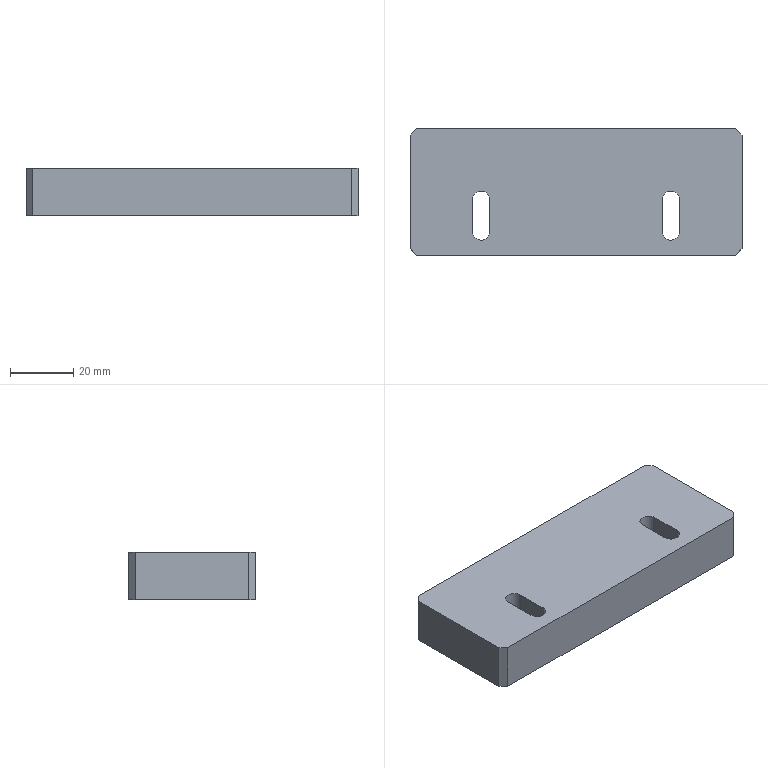Part | STEP file | PN_0019 | 1 solid | 34 faces | box 105 x 40 x 15 mm | volume 59951 mm3 | plane 14 | cylinder 12 | cone 8 | commonest cylinder face diameters 4 x4 4.2 x4 5.5 x4